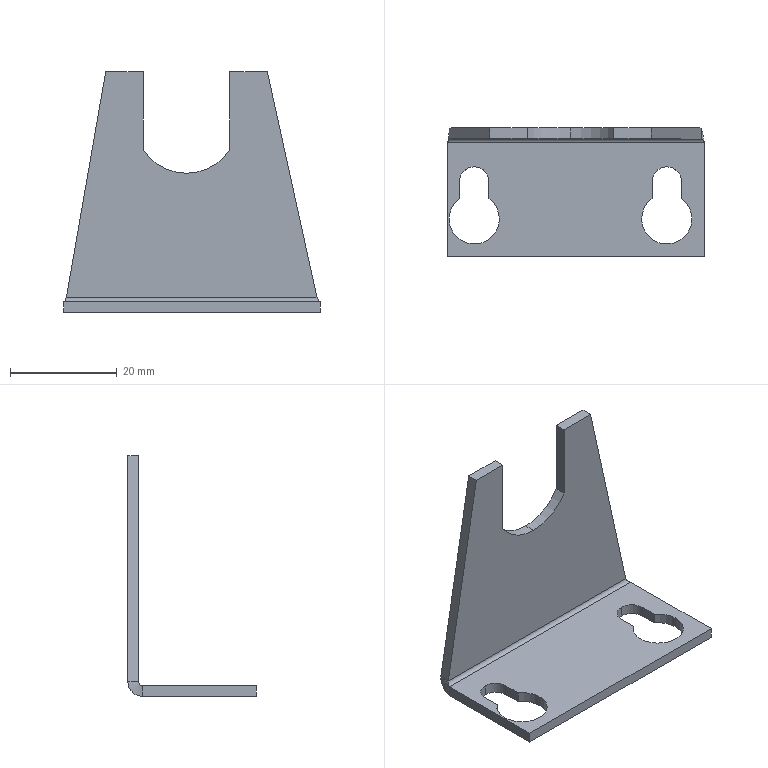Part | SolidWorks | features BaseBody 1 | 1 solid | 29 faces | box 47.946 x 24 x 45 mm | volume 4600 mm3 | plane 17 | cylinder 10 | spline 2 | commonest cylinder face diameters 5.5 x4 9.4 x2 19.08 x2 1.473 x1 5.473 x1
STEP:
#1=CARTESIAN_POINT('',(0.,2.,-10.682));
#2=VERTEX_POINT('',#1);
#3=CARTESIAN_POINT('',(8.1,2.,-6.182));
#4=VERTEX_POINT('',#3);
#5=CARTESIAN_POINT('',(0.,2.,-1.142));
#6=DIRECTION('',(0.,-1.,0.));
#7=DIRECTION('',(0.,0.,-1.));
#8=AXIS2_PLACEMENT_3D('',#5,#6,#7);
#9=CIRCLE('',#8,9.54);
#10=EDGE_CURVE('',#2,#4,#9,.T.);
#11=ORIENTED_EDGE('',*,*,#10,.F.);
#12=CARTESIAN_POINT('',(0.,0.,-10.682));
#13=VERTEX_POINT('',#12);
#14=CARTESIAN_POINT('',(0.,2.,-10.682));
#15=DIRECTION('',(0.,-1.,0.));
#16=VECTOR('',#15,1000.);
#17=LINE('',#14,#16);
#18=EDGE_CURVE('',#2,#13,#17,.T.);
#19=ORIENTED_EDGE('',*,*,#18,.T.);
#20=CARTESIAN_POINT('',(8.1,0.,-6.182));
#21=VERTEX_POINT('',#20);
#22=CARTESIAN_POINT('',(0.,0.,-1.142));
#23=DIRECTION('',(0.,1.,0.));
#24=DIRECTION('',(0.,0.,-1.));
#25=AXIS2_PLACEMENT_3D('',#22,#23,#24);
#26=CIRCLE('',#25,9.54);
#27=EDGE_CURVE('',#21,#13,#26,.T.);
#28=ORIENTED_EDGE('',*,*,#27,.F.);
#29=CARTESIAN_POINT('',(8.1,2.,-6.182));
#30=DIRECTION('',(0.,-1.,0.));
#31=VECTOR('',#30,1000.);
#32=LINE('',#29,#31);
#33=EDGE_CURVE('',#4,#21,#32,.T.);
#34=ORIENTED_EDGE('',*,*,#33,.F.);
#35=EDGE_LOOP('',(#11,#19,#28,#34));
#36=FACE_OUTER_BOUND('',#35,.T.);
#37=CARTESIAN_POINT('',(0.,2.,-1.142));
#38=DIRECTION('',(0.,-1.,0.));
#39=DIRECTION('',(0.,0.,-1.));
#40=AXIS2_PLACEMENT_3D('',#37,#38,#39);
#41=CYLINDRICAL_SURFACE('',#40,9.54);
#42=ADVANCED_FACE('',(#36),#41,.F.);
#43=CARTESIAN_POINT('',(-15.25,-8.,-34.682));
#44=VERTEX_POINT('',#43);
#45=CARTESIAN_POINT('',(-18.,-5.25,-34.682));
#46=VERTEX_POINT('',#45);
#47=CARTESIAN_POINT('',(-18.,-8.,-34.682));
#48=DIRECTION('',(0.,0.,1.));
#49=DIRECTION('',(0.,1.,0.));
#50=AXIS2_PLACEMENT_3D('',#47,#48,#49);
#51=CIRCLE('',#50,2.75);
#52=EDGE_CURVE('',#44,#46,#51,.T.);
#53=ORIENTED_EDGE('',*,*,#52,.T.);
#54=CARTESIAN_POINT('',(-18.,-5.25,-36.682));
#55=VERTEX_POINT('',#54);
#56=CARTESIAN_POINT('',(-18.,-5.25,-26.682));
#57=DIRECTION('',(0.,0.,-1.));
#58=VECTOR('',#57,1000.);
#59=LINE('',#56,#58);
#60=EDGE_CURVE('',#46,#55,#59,.T.);
#61=ORIENTED_EDGE('',*,*,#60,.T.);
#62=CARTESIAN_POINT('',(-15.25,-8.,-36.682));
#63=VERTEX_POINT('',#62);
#64=CARTESIAN_POINT('',(-18.,-8.,-36.682));
#65=DIRECTION('',(0.,0.,1.));
#66=DIRECTION('',(0.,1.,0.));
#67=AXIS2_PLACEMENT_3D('',#64,#65,#66);
#68=CIRCLE('',#67,2.75);
#69=EDGE_CURVE('',#63,#55,#68,.T.);
#70=ORIENTED_EDGE('',*,*,#69,.F.);
#71=CARTESIAN_POINT('',(-15.25,-8.,-26.682));
#72=DIRECTION('',(0.,0.,1.));
#73=VECTOR('',#72,1000.);
#74=LINE('',#71,#73);
#75=EDGE_CURVE('',#63,#44,#74,.T.);
#76=ORIENTED_EDGE('',*,*,#75,.T.);
#77=EDGE_LOOP('',(#53,#61,#70,#76));
#78=FACE_OUTER_BOUND('',#77,.T.);
#79=CARTESIAN_POINT('',(-18.,-8.,-26.682));
#80=DIRECTION('',(0.,0.,-1.));
#81=DIRECTION('',(0.,1.,0.));
#82=AXIS2_PLACEMENT_3D('',#79,#80,#81);
#83=CYLINDRICAL_SURFACE('',#82,2.75);
#84=ADVANCED_FACE('',(#78),#83,.F.);
#85=CARTESIAN_POINT('',(20.75,-8.,-34.682));
#86=VERTEX_POINT('',#85);
#87=CARTESIAN_POINT('',(18.,-5.25,-34.682));
#88=VERTEX_POINT('',#87);
#89=CARTESIAN_POINT('',(18.,-8.,-34.682));
#90=DIRECTION('',(0.,0.,1.));
#91=DIRECTION('',(0.,1.,0.));
#92=AXIS2_PLACEMENT_3D('',#89,#90,#91);
#93=CIRCLE('',#92,2.75);
#94=EDGE_CURVE('',#86,#88,#93,.T.);
#95=ORIENTED_EDGE('',*,*,#94,.T.);
#96=CARTESIAN_POINT('',(18.,-5.25,-36.682));
#97=VERTEX_POINT('',#96);
#98=CARTESIAN_POINT('',(18.,-5.25,-26.682));
#99=DIRECTION('',(0.,0.,-1.));
#100=VECTOR('',#99,1000.);
#101=LINE('',#98,#100);
#102=EDGE_CURVE('',#88,#97,#101,.T.);
#103=ORIENTED_EDGE('',*,*,#102,.T.);
#104=CARTESIAN_POINT('',(20.75,-8.,-36.682));
#105=VERTEX_POINT('',#104);
#106=CARTESIAN_POINT('',(18.,-8.,-36.682));
#107=DIRECTION('',(0.,0.,1.));
#108=DIRECTION('',(0.,1.,0.));
#109=AXIS2_PLACEMENT_3D('',#106,#107,#108);
#110=CIRCLE('',#109,2.75);
#111=EDGE_CURVE('',#105,#97,#110,.T.);
#112=ORIENTED_EDGE('',*,*,#111,.F.);
#113=CARTESIAN_POINT('',(20.75,-8.,-26.682));
#114=DIRECTION('',(0.,0.,1.));
#115=VECTOR('',#114,1000.);
#116=LINE('',#113,#115);
#117=EDGE_CURVE('',#105,#86,#116,.T.);
#118=ORIENTED_EDGE('',*,*,#117,.T.);
#119=EDGE_LOOP('',(#95,#103,#112,#118));
#120=FACE_OUTER_BOUND('',#119,.T.);
#121=CARTESIAN_POINT('',(18.,-8.,-26.682));
#122=DIRECTION('',(0.,0.,-1.));
#123=DIRECTION('',(0.,1.,0.));
#124=AXIS2_PLACEMENT_3D('',#121,#122,#123);
#125=CYLINDRICAL_SURFACE('',#124,2.75);
#126=ADVANCED_FACE('',(#120),#125,.F.);
#127=ORIENTED_EDGE('',*,*,#111,.T.);
#128=CARTESIAN_POINT('',(15.25,-8.,-36.682));
#129=VERTEX_POINT('',#128);
#130=CARTESIAN_POINT('',(18.,-8.,-36.682));
#131=DIRECTION('',(0.,0.,1.));
#132=DIRECTION('',(0.,1.,0.));
#133=AXIS2_PLACEMENT_3D('',#130,#131,#132);
#134=CIRCLE('',#133,2.75);
#135=EDGE_CURVE('',#97,#129,#134,.T.);
#136=ORIENTED_EDGE('',*,*,#135,.T.);
#137=CARTESIAN_POINT('',(15.25,-11.189,-36.682));
#138=VERTEX_POINT('',#137);
#139=CARTESIAN_POINT('',(15.25,-8.,-36.682));
#140=DIRECTION('',(0.,-1.,0.));
#141=VECTOR('',#140,1000.);
#142=LINE('',#139,#141);
#143=EDGE_CURVE('',#129,#138,#142,.T.);
#144=ORIENTED_EDGE('',*,*,#143,.T.);
#145=CARTESIAN_POINT('',(20.75,-11.189,-36.682));
#146=VERTEX_POINT('',#145);
#147=CARTESIAN_POINT('',(18.,-15.,-36.682));
#148=DIRECTION('',(0.,0.,1.));
#149=DIRECTION('',(0.,1.,0.));
#150=AXIS2_PLACEMENT_3D('',#147,#148,#149);
#151=CIRCLE('',#150,4.7);
#152=EDGE_CURVE('',#138,#146,#151,.T.);
#153=ORIENTED_EDGE('',*,*,#152,.T.);
#154=CARTESIAN_POINT('',(20.75,-8.,-36.682));
#155=DIRECTION('',(0.,1.,0.));
#156=VECTOR('',#155,1000.);
#157=LINE('',#154,#156);
#158=EDGE_CURVE('',#146,#105,#157,.T.);
#159=ORIENTED_EDGE('',*,*,#158,.T.);
#160=EDGE_LOOP('',(#127,#136,#144,#153,#159));
#161=FACE_BOUND('',#160,.T.);
#162=ORIENTED_EDGE('',*,*,#69,.T.);
#163=CARTESIAN_POINT('',(-20.75,-8.,-36.682));
#164=VERTEX_POINT('',#163);
#165=CARTESIAN_POINT('',(-18.,-8.,-36.682));
#166=DIRECTION('',(0.,0.,1.));
#167=DIRECTION('',(0.,1.,0.));
#168=AXIS2_PLACEMENT_3D('',#165,#166,#167);
#169=CIRCLE('',#168,2.75);
#170=EDGE_CURVE('',#55,#164,#169,.T.);
#171=ORIENTED_EDGE('',*,*,#170,.T.);
#172=CARTESIAN_POINT('',(-20.75,-11.189,-36.682));
#173=VERTEX_POINT('',#172);
#174=CARTESIAN_POINT('',(-20.75,-8.,-36.682));
#175=DIRECTION('',(0.,-1.,0.));
#176=VECTOR('',#175,1000.);
#177=LINE('',#174,#176);
#178=EDGE_CURVE('',#164,#173,#177,.T.);
#179=ORIENTED_EDGE('',*,*,#178,.T.);
#180=CARTESIAN_POINT('',(-15.25,-11.189,-36.682));
#181=VERTEX_POINT('',#180);
#182=CARTESIAN_POINT('',(-18.,-15.,-36.682));
#183=DIRECTION('',(0.,0.,1.));
#184=DIRECTION('',(0.,1.,0.));
#185=AXIS2_PLACEMENT_3D('',#182,#183,#184);
#186=CIRCLE('',#185,4.7);
#187=EDGE_CURVE('',#173,#181,#186,.T.);
#188=ORIENTED_EDGE('',*,*,#187,.T.);
#189=CARTESIAN_POINT('',(-15.25,-8.,-36.682));
#190=DIRECTION('',(0.,1.,0.));
#191=VECTOR('',#190,1000.);
#192=LINE('',#189,#191);
#193=EDGE_CURVE('',#181,#63,#192,.T.);
#194=ORIENTED_EDGE('',*,*,#193,.T.);
#195=EDGE_LOOP('',(#162,#171,#179,#188,#194));
#196=FACE_BOUND('',#195,.T.);
#197=CARTESIAN_POINT('',(25.,-22.,-36.682));
#198=VERTEX_POINT('',#197);
#199=CARTESIAN_POINT('',(25.,-0.7366,-36.682));
#200=VERTEX_POINT('',#199);
#201=CARTESIAN_POINT('',(25.,0.,-36.682));
#202=DIRECTION('',(0.,1.,0.));
#203=VECTOR('',#202,1000.);
#204=LINE('',#201,#203);
#205=EDGE_CURVE('',#198,#200,#204,.T.);
#206=ORIENTED_EDGE('',*,*,#205,.F.);
#207=CARTESIAN_POINT('',(-22.946,-22.,-36.682));
#208=VERTEX_POINT('',#207);
#209=CARTESIAN_POINT('',(25.,-22.,-36.682));
#210=DIRECTION('',(1.,0.,0.));
#211=VECTOR('',#210,1000.);
#212=LINE('',#209,#211);
#213=EDGE_CURVE('',#208,#198,#212,.T.);
#214=ORIENTED_EDGE('',*,*,#213,.F.);
#215=CARTESIAN_POINT('',(-22.946,-0.7366,-36.682));
#216=VERTEX_POINT('',#215);
#217=CARTESIAN_POINT('',(-22.946,-22.,-36.682));
#218=DIRECTION('',(0.,-1.,0.));
#219=VECTOR('',#218,1000.);
#220=LINE('',#217,#219);
#221=EDGE_CURVE('',#216,#208,#220,.T.);
#222=ORIENTED_EDGE('',*,*,#221,.F.);
#223=CARTESIAN_POINT('',(25.,-0.7366,-36.682));
#224=DIRECTION('',(-1.,0.,0.));
#225=VECTOR('',#224,1000.);
#226=LINE('',#223,#225);
#227=EDGE_CURVE('',#200,#216,#226,.T.);
#228=ORIENTED_EDGE('',*,*,#227,.F.);
#229=EDGE_LOOP('',(#206,#214,#222,#228));
#230=FACE_OUTER_BOUND('',#229,.T.);
#231=CARTESIAN_POINT('',(25.,0.,-36.682));
#232=DIRECTION('',(0.,0.,-1.));
#233=DIRECTION('',(-1.,0.,0.));
#234=AXIS2_PLACEMENT_3D('',#231,#232,#233);
#235=PLANE('',#234);
#236=ADVANCED_FACE('',(#161,#196,#230),#235,.T.);
#237=ORIENTED_EDGE('',*,*,#143,.F.);
#238=CARTESIAN_POINT('',(15.25,-8.,-34.682));
#239=VERTEX_POINT('',#238);
#240=CARTESIAN_POINT('',(15.25,-8.,-26.682));
#241=DIRECTION('',(0.,0.,-1.));
#242=VECTOR('',#241,1000.);
#243=LINE('',#240,#242);
#244=EDGE_CURVE('',#239,#129,#243,.T.);
#245=ORIENTED_EDGE('',*,*,#244,.F.);
#246=CARTESIAN_POINT('',(15.25,-11.189,-34.682));
#247=VERTEX_POINT('',#246);
#248=CARTESIAN_POINT('',(15.25,0.,-34.682));
#249=DIRECTION('',(0.,-1.,0.));
#250=VECTOR('',#249,1000.);
#251=LINE('',#248,#250);
#252=EDGE_CURVE('',#239,#247,#251,.T.);
#253=ORIENTED_EDGE('',*,*,#252,.T.);
#254=CARTESIAN_POINT('',(15.25,-11.189,-26.682));
#255=DIRECTION('',(0.,0.,-1.));
#256=VECTOR('',#255,1000.);
#257=LINE('',#254,#256);
#258=EDGE_CURVE('',#247,#138,#257,.T.);
#259=ORIENTED_EDGE('',*,*,#258,.T.);
#260=EDGE_LOOP('',(#237,#245,#253,#259));
#261=FACE_OUTER_BOUND('',#260,.T.);
#262=CARTESIAN_POINT('',(15.25,-8.,-26.682));
#263=DIRECTION('',(-1.,0.,0.));
#264=DIRECTION('',(0.,1.,0.));
#265=AXIS2_PLACEMENT_3D('',#262,#263,#264);
#266=PLANE('',#265);
#267=ADVANCED_FACE('',(#261),#266,.F.);
#268=ORIENTED_EDGE('',*,*,#152,.F.);
#269=ORIENTED_EDGE('',*,*,#258,.F.);
#270=CARTESIAN_POINT('',(20.75,-11.189,-34.682));
#271=VERTEX_POINT('',#270);
#272=CARTESIAN_POINT('',(18.,-15.,-34.682));
#273=DIRECTION('',(0.,0.,1.));
#274=DIRECTION('',(0.,1.,0.));
#275=AXIS2_PLACEMENT_3D('',#272,#273,#274);
#276=CIRCLE('',#275,4.7);
#277=EDGE_CURVE('',#247,#271,#276,.T.);
#278=ORIENTED_EDGE('',*,*,#277,.T.);
#279=CARTESIAN_POINT('',(20.75,-11.189,-26.682));
#280=DIRECTION('',(0.,0.,-1.));
#281=VECTOR('',#280,1000.);
#282=LINE('',#279,#281);
#283=EDGE_CURVE('',#271,#146,#282,.T.);
#284=ORIENTED_EDGE('',*,*,#283,.T.);
#285=EDGE_LOOP('',(#268,#269,#278,#284));
#286=FACE_OUTER_BOUND('',#285,.T.);
#287=CARTESIAN_POINT('',(18.,-15.,-26.682));
#288=DIRECTION('',(0.,0.,-1.));
#289=DIRECTION('',(0.,1.,0.));
#290=AXIS2_PLACEMENT_3D('',#287,#288,#289);
#291=CYLINDRICAL_SURFACE('',#290,4.7);
#292=ADVANCED_FACE('',(#286),#291,.F.);
#293=ORIENTED_EDGE('',*,*,#158,.F.);
#294=ORIENTED_EDGE('',*,*,#283,.F.);
#295=CARTESIAN_POINT('',(20.75,0.,-34.682));
#296=DIRECTION('',(0.,1.,0.));
#297=VECTOR('',#296,1000.);
#298=LINE('',#295,#297);
#299=EDGE_CURVE('',#271,#86,#298,.T.);
#300=ORIENTED_EDGE('',*,*,#299,.T.);
#301=ORIENTED_EDGE('',*,*,#117,.F.);
#302=EDGE_LOOP('',(#293,#294,#300,#301));
#303=FACE_OUTER_BOUND('',#302,.T.);
#304=CARTESIAN_POINT('',(20.75,-8.,-26.682));
#305=DIRECTION('',(1.,0.,0.));
#306=DIRECTION('',(0.,0.,-1.));
#307=AXIS2_PLACEMENT_3D('',#304,#305,#306);
#308=PLANE('',#307);
#309=ADVANCED_FACE('',(#303),#308,.F.);
#310=ORIENTED_EDGE('',*,*,#178,.F.);
#311=CARTESIAN_POINT('',(-20.75,-8.,-34.682));
#312=VERTEX_POINT('',#311);
#313=CARTESIAN_POINT('',(-20.75,-8.,-26.682));
#314=DIRECTION('',(0.,0.,-1.));
#315=VECTOR('',#314,1000.);
#316=LINE('',#313,#315);
#317=EDGE_CURVE('',#312,#164,#316,.T.);
#318=ORIENTED_EDGE('',*,*,#317,.F.);
#319=CARTESIAN_POINT('',(-20.75,-11.189,-34.682));
#320=VERTEX_POINT('',#319);
#321=CARTESIAN_POINT('',(-20.75,0.,-34.682));
#322=DIRECTION('',(0.,-1.,0.));
#323=VECTOR('',#322,1000.);
#324=LINE('',#321,#323);
#325=EDGE_CURVE('',#312,#320,#324,.T.);
#326=ORIENTED_EDGE('',*,*,#325,.T.);
#327=CARTESIAN_POINT('',(-20.75,-11.189,-26.682));
#328=DIRECTION('',(0.,0.,-1.));
#329=VECTOR('',#328,1000.);
#330=LINE('',#327,#329);
#331=EDGE_CURVE('',#320,#173,#330,.T.);
#332=ORIENTED_EDGE('',*,*,#331,.T.);
#333=EDGE_LOOP('',(#310,#318,#326,#332));
#334=FACE_OUTER_BOUND('',#333,.T.);
#335=CARTESIAN_POINT('',(-20.75,-8.,-26.682));
#336=DIRECTION('',(-1.,0.,0.));
#337=DIRECTION('',(0.,1.,0.));
#338=AXIS2_PLACEMENT_3D('',#335,#336,#337);
#339=PLANE('',#338);
#340=ADVANCED_FACE('',(#334),#339,.F.);
#341=ORIENTED_EDGE('',*,*,#187,.F.);
#342=ORIENTED_EDGE('',*,*,#331,.F.);
#343=CARTESIAN_POINT('',(-15.25,-11.189,-34.682));
#344=VERTEX_POINT('',#343);
#345=CARTESIAN_POINT('',(-18.,-15.,-34.682));
#346=DIRECTION('',(0.,0.,1.));
#347=DIRECTION('',(0.,1.,0.));
#348=AXIS2_PLACEMENT_3D('',#345,#346,#347);
#349=CIRCLE('',#348,4.7);
#350=EDGE_CURVE('',#320,#344,#349,.T.);
#351=ORIENTED_EDGE('',*,*,#350,.T.);
#352=CARTESIAN_POINT('',(-15.25,-11.189,-26.682));
#353=DIRECTION('',(0.,0.,-1.));
#354=VECTOR('',#353,1000.);
#355=LINE('',#352,#354);
#356=EDGE_CURVE('',#344,#181,#355,.T.);
#357=ORIENTED_EDGE('',*,*,#356,.T.);
#358=EDGE_LOOP('',(#341,#342,#351,#357));
#359=FACE_OUTER_BOUND('',#358,.T.);
#360=CARTESIAN_POINT('',(-18.,-15.,-26.682));
#361=DIRECTION('',(0.,0.,-1.));
#362=DIRECTION('',(0.,1.,0.));
#363=AXIS2_PLACEMENT_3D('',#360,#361,#362);
#364=CYLINDRICAL_SURFACE('',#363,4.7);
#365=ADVANCED_FACE('',(#359),#364,.F.);
#366=ORIENTED_EDGE('',*,*,#193,.F.);
#367=ORIENTED_EDGE('',*,*,#356,.F.);
#368=CARTESIAN_POINT('',(-15.25,0.,-34.682));
#369=DIRECTION('',(0.,1.,0.));
#370=VECTOR('',#369,1000.);
#371=LINE('',#368,#370);
#372=EDGE_CURVE('',#344,#44,#371,.T.);
#373=ORIENTED_EDGE('',*,*,#372,.T.);
#374=ORIENTED_EDGE('',*,*,#75,.F.);
#375=EDGE_LOOP('',(#366,#367,#373,#374));
#376=FACE_OUTER_BOUND('',#375,.T.);
#377=CARTESIAN_POINT('',(-15.25,-8.,-26.682));
#378=DIRECTION('',(1.,0.,0.));
#379=DIRECTION('',(0.,0.,-1.));
#380=AXIS2_PLACEMENT_3D('',#377,#378,#379);
#381=PLANE('',#380);
#382=ADVANCED_FACE('',(#376),#381,.F.);
#383=ORIENTED_EDGE('',*,*,#213,.T.);
#384=CARTESIAN_POINT('',(25.,-22.,-34.682));
#385=VERTEX_POINT('',#384);
#386=CARTESIAN_POINT('',(25.,-22.,-36.682));
#387=DIRECTION('',(0.,0.,-1.));
#388=VECTOR('',#387,1000.);
#389=LINE('',#386,#388);
#390=EDGE_CURVE('',#385,#198,#389,.T.);
#391=ORIENTED_EDGE('',*,*,#390,.F.);
#392=CARTESIAN_POINT('',(-22.946,-22.,-34.682));
#393=VERTEX_POINT('',#392);
#394=CARTESIAN_POINT('',(25.,-22.,-34.682));
#395=DIRECTION('',(-1.,0.,0.));
#396=VECTOR('',#395,1000.);
#397=LINE('',#394,#396);
#398=EDGE_CURVE('',#385,#393,#397,.T.);
#399=ORIENTED_EDGE('',*,*,#398,.T.);
#400=CARTESIAN_POINT('',(-22.946,-22.,-36.682));
#401=DIRECTION('',(0.,0.,1.));
#402=VECTOR('',#401,1000.);
#403=LINE('',#400,#402);
#404=EDGE_CURVE('',#208,#393,#403,.T.);
#405=ORIENTED_EDGE('',*,*,#404,.F.);
#406=EDGE_LOOP('',(#383,#391,#399,#405));
#407=FACE_OUTER_BOUND('',#406,.T.);
#408=CARTESIAN_POINT('',(25.,-22.,-36.682));
#409=DIRECTION('',(0.,-1.,0.));
#410=DIRECTION('',(0.,0.,-1.));
#411=AXIS2_PLACEMENT_3D('',#408,#409,#410);
#412=PLANE('',#411);
#413=ADVANCED_FACE('',(#407),#412,.T.);
#414=ORIENTED_EDGE('',*,*,#221,.T.);
#415=ORIENTED_EDGE('',*,*,#404,.T.);
#416=CARTESIAN_POINT('',(-22.946,-0.7366,-34.682));
#417=VERTEX_POINT('',#416);
#418=CARTESIAN_POINT('',(-22.946,0.,-34.682));
#419=DIRECTION('',(0.,1.,0.));
#420=VECTOR('',#419,1000.);
#421=LINE('',#418,#420);
#422=EDGE_CURVE('',#393,#417,#421,.T.);
#423=ORIENTED_EDGE('',*,*,#422,.T.);
#424=CARTESIAN_POINT('',(-22.946,-0.7366,-35.682));
#425=DIRECTION('',(0.,0.,-1.));
#426=VECTOR('',#425,1000.);
#427=LINE('',#424,#426);
#428=EDGE_CURVE('',#417,#216,#427,.T.);
#429=ORIENTED_EDGE('',*,*,#428,.T.);
#430=EDGE_LOOP('',(#414,#415,#423,#429));
#431=FACE_OUTER_BOUND('',#430,.T.);
#432=CARTESIAN_POINT('',(-22.946,-22.,-36.682));
#433=DIRECTION('',(-1.,0.,0.));
#434=DIRECTION('',(0.,1.,0.));
#435=AXIS2_PLACEMENT_3D('',#432,#433,#434);
#436=PLANE('',#435);
#437=ADVANCED_FACE('',(#431),#436,.T.);
#438=CARTESIAN_POINT('',(25.,-0.7366,-34.682));
#439=VERTEX_POINT('',#438);
#440=CARTESIAN_POINT('',(25.,0.,-34.682));
#441=DIRECTION('',(0.,-1.,0.));
#442=VECTOR('',#441,1000.);
#443=LINE('',#440,#442);
#444=EDGE_CURVE('',#439,#385,#443,.T.);
#445=ORIENTED_EDGE('',*,*,#444,.T.);
#446=ORIENTED_EDGE('',*,*,#390,.T.);
#447=ORIENTED_EDGE('',*,*,#205,.T.);
#448=CARTESIAN_POINT('',(25.,-0.7366,-35.682));
#449=DIRECTION('',(0.,0.,1.));
#450=VECTOR('',#449,1000.);
#451=LINE('',#448,#450);
#452=EDGE_CURVE('',#200,#439,#451,.T.);
#453=ORIENTED_EDGE('',*,*,#452,.T.);
#454=EDGE_LOOP('',(#445,#446,#447,#453));
#455=FACE_OUTER_BOUND('',#454,.T.);
#456=CARTESIAN_POINT('',(25.,0.,-36.682));
#457=DIRECTION('',(1.,0.,0.));
#458=DIRECTION('',(0.,0.,-1.));
#459=AXIS2_PLACEMENT_3D('',#456,#457,#458);
#460=PLANE('',#459);
#461=ADVANCED_FACE('',(#455),#460,.T.);
#462=ORIENTED_EDGE('',*,*,#227,.T.);
#463=CARTESIAN_POINT('',(-22.469,2.,-33.946));
#464=VERTEX_POINT('',#463);
#465=CARTESIAN_POINT('',(-22.946,-0.7366,-36.682));
#466=CARTESIAN_POINT('',(-22.906,-0.3784,-36.682));
#467=CARTESIAN_POINT('',(-22.867,-0.0203,-36.611));
#468=CARTESIAN_POINT('',(-22.787,0.6416,-36.337));
#469=CARTESIAN_POINT('',(-22.747,0.9452,-36.134));
#470=CARTESIAN_POINT('',(-22.668,1.452,-35.628));
#471=CARTESIAN_POINT('',(-22.628,1.655,-35.324));
#472=CARTESIAN_POINT('',(-22.549,1.929,-34.662));
#473=CARTESIAN_POINT('',(-22.509,2.,-34.304));
#474=CARTESIAN_POINT('',(-22.469,2.,-33.946));
#475=B_SPLINE_CURVE_WITH_KNOTS('',3,(#465,#466,#467,#468,#469,#470,#471,#472,#473,#474),.UNSPECIFIED.,.F.,.F.,(4,2,2,2,4),(0.,0.25,0.5,0.75,1.),.UNSPECIFIED.);
#476=EDGE_CURVE('',#216,#464,#475,.T.);
#477=ORIENTED_EDGE('',*,*,#476,.T.);
#478=CARTESIAN_POINT('',(24.398,2.,-33.946));
#479=VERTEX_POINT('',#478);
#480=CARTESIAN_POINT('',(0.,2.,-33.946));
#481=DIRECTION('',(1.,0.,0.));
#482=VECTOR('',#481,1000.);
#483=LINE('',#480,#482);
#484=EDGE_CURVE('',#464,#479,#483,.T.);
#485=ORIENTED_EDGE('',*,*,#484,.T.);
#486=CARTESIAN_POINT('',(24.398,2.,-33.946));
#487=CARTESIAN_POINT('',(24.449,2.,-34.307));
#488=CARTESIAN_POINT('',(24.498,1.93,-34.657));
#489=CARTESIAN_POINT('',(24.573,1.724,-35.158));
#490=CARTESIAN_POINT('',(24.598,1.64,-35.315));
#491=CARTESIAN_POINT('',(24.648,1.442,-35.612));
#492=CARTESIAN_POINT('',(24.674,1.327,-35.753));
#493=CARTESIAN_POINT('',(24.724,1.073,-36.006));
#494=CARTESIAN_POINT('',(24.749,0.9356,-36.119));
#495=CARTESIAN_POINT('',(24.799,0.6384,-36.319));
#496=CARTESIAN_POINT('',(24.824,0.4778,-36.405));
#497=CARTESIAN_POINT('',(24.899,-0.01677,-36.61));
#498=CARTESIAN_POINT('',(24.949,-0.375,-36.682));
#499=CARTESIAN_POINT('',(25.,-0.7366,-36.682));
#500=B_SPLINE_CURVE_WITH_KNOTS('',3,(#486,#487,#488,#489,#490,#491,#492,#493,#494,#495,#496,#497,#498,#499),.UNSPECIFIED.,.F.,.F.,(4,2,2,2,2,2,4),(0.,0.001076,0.001614,0.002152,0.00269,0.003228,0.004304),.UNSPECIFIED.);
#501=EDGE_CURVE('',#479,#200,#500,.T.);
#502=ORIENTED_EDGE('',*,*,#501,.T.);
#503=EDGE_LOOP('',(#462,#477,#485,#502));
#504=FACE_OUTER_BOUND('',#503,.T.);
#505=CARTESIAN_POINT('',(25.,-0.7366,-33.946));
#506=DIRECTION('',(1.,0.,0.));
#507=DIRECTION('',(0.,0.,-1.));
#508=AXIS2_PLACEMENT_3D('',#505,#506,#507);
#509=CYLINDRICAL_SURFACE('',#508,2.737);
#510=ADVANCED_FACE('',(#504),#509,.T.);
#511=CARTESIAN_POINT('',(-22.469,0.,-33.946));
#512=VERTEX_POINT('',#511);
#513=CARTESIAN_POINT('',(-22.469,0.,-33.946));
#514=CARTESIAN_POINT('',(-22.549,0.,-34.139));
#515=CARTESIAN_POINT('',(-22.628,-0.07939,-34.33));
#516=CARTESIAN_POINT('',(-22.787,-0.3521,-34.603));
#517=CARTESIAN_POINT('',(-22.867,-0.5438,-34.682));
#518=CARTESIAN_POINT('',(-22.946,-0.7366,-34.682));
#519=B_SPLINE_CURVE_WITH_KNOTS('',3,(#513,#514,#515,#516,#517,#518),.UNSPECIFIED.,.F.,.F.,(4,2,4),(0.,0.5,1.),.UNSPECIFIED.);
#520=EDGE_CURVE('',#512,#417,#519,.T.);
#521=ORIENTED_EDGE('',*,*,#520,.F.);
#522=CARTESIAN_POINT('',(-22.469,2.,-33.946));
#523=DIRECTION('',(0.,1.,0.));
#524=VECTOR('',#523,1000.);
#525=LINE('',#522,#524);
#526=EDGE_CURVE('',#512,#464,#525,.T.);
#527=ORIENTED_EDGE('',*,*,#526,.T.);
#528=ORIENTED_EDGE('',*,*,#476,.F.);
#529=ORIENTED_EDGE('',*,*,#428,.F.);
#530=EDGE_LOOP('',(#521,#527,#528,#529));
#531=FACE_OUTER_BOUND('',#530,.T.);
#532=CARTESIAN_POINT('',(-22.469,2.02,-33.946));
#533=CARTESIAN_POINT('',(-22.509,2.02,-34.307));
#534=CARTESIAN_POINT('',(-22.549,1.948,-34.667));
#535=CARTESIAN_POINT('',(-22.628,1.672,-35.334));
#536=CARTESIAN_POINT('',(-22.668,1.468,-35.64));
#537=CARTESIAN_POINT('',(-22.747,0.9575,-36.15));
#538=CARTESIAN_POINT('',(-22.787,0.6517,-36.354));
#539=CARTESIAN_POINT('',(-22.867,-0.01507,-36.631));
#540=CARTESIAN_POINT('',(-22.906,-0.3757,-36.702));
#541=CARTESIAN_POINT('',(-22.946,-0.7366,-36.702));
#542=CARTESIAN_POINT('',(-22.469,2.,-33.946));
#543=CARTESIAN_POINT('',(-22.509,2.,-34.304));
#544=CARTESIAN_POINT('',(-22.549,1.929,-34.662));
#545=CARTESIAN_POINT('',(-22.628,1.655,-35.324));
#546=CARTESIAN_POINT('',(-22.668,1.452,-35.628));
#547=CARTESIAN_POINT('',(-22.747,0.9452,-36.134));
#548=CARTESIAN_POINT('',(-22.787,0.6416,-36.337));
#549=CARTESIAN_POINT('',(-22.867,-0.0203,-36.611));
#550=CARTESIAN_POINT('',(-22.906,-0.3783,-36.682));
#551=CARTESIAN_POINT('',(-22.946,-0.7366,-36.682));
#552=CARTESIAN_POINT('',(-22.469,0.,-33.946));
#553=CARTESIAN_POINT('',(-22.509,0.,-34.042));
#554=CARTESIAN_POINT('',(-22.549,-0.01917,-34.139));
#555=CARTESIAN_POINT('',(-22.628,-0.09297,-34.317));
#556=CARTESIAN_POINT('',(-22.668,-0.1476,-34.398));
#557=CARTESIAN_POINT('',(-22.747,-0.2839,-34.535));
#558=CARTESIAN_POINT('',(-22.787,-0.3656,-34.589));
#559=CARTESIAN_POINT('',(-22.867,-0.5438,-34.663));
#560=CARTESIAN_POINT('',(-22.906,-0.6402,-34.682));
#561=CARTESIAN_POINT('',(-22.946,-0.7366,-34.682));
#562=CARTESIAN_POINT('',(-22.469,-0.0202,-33.946));
#563=CARTESIAN_POINT('',(-22.509,-0.0202,-34.04));
#564=CARTESIAN_POINT('',(-22.549,-0.03885,-34.133));
#565=CARTESIAN_POINT('',(-22.628,-0.1106,-34.307));
#566=CARTESIAN_POINT('',(-22.668,-0.1637,-34.386));
#567=CARTESIAN_POINT('',(-22.747,-0.2963,-34.519));
#568=CARTESIAN_POINT('',(-22.787,-0.3758,-34.572));
#569=CARTESIAN_POINT('',(-22.867,-0.5491,-34.644));
#570=CARTESIAN_POINT('',(-22.906,-0.6428,-34.662));
#571=CARTESIAN_POINT('',(-22.946,-0.7366,-34.662));
#572=B_SPLINE_SURFACE_WITH_KNOTS('',1,3,((#532,#533,#534,#535,#536,#537,#538,#539,#540,#541),(#542,#543,#544,#545,#546,#547,#548,#549,#550,#551),(#552,#553,#554,#555,#556,#557,#558,#559,#560,#561),(#562,#563,#564,#565,#566,#567,#568,#569,#570,#571)),.UNSPECIFIED.,.F.,.F.,.F.,(2,1,1,2),(4,2,2,2,4),(-0.01,0.,1.,1.01),(0.,0.25,0.5,0.75,1.),.UNSPECIFIED.);
#573=ADVANCED_FACE('',(#531),#572,.F.);
#574=ORIENTED_EDGE('',*,*,#277,.F.);
#575=ORIENTED_EDGE('',*,*,#252,.F.);
#576=CARTESIAN_POINT('',(18.,-8.,-34.682));
#577=DIRECTION('',(0.,0.,1.));
#578=DIRECTION('',(0.,1.,0.));
#579=AXIS2_PLACEMENT_3D('',#576,#577,#578);
#580=CIRCLE('',#579,2.75);
#581=EDGE_CURVE('',#88,#239,#580,.T.);
#582=ORIENTED_EDGE('',*,*,#581,.F.);
#583=ORIENTED_EDGE('',*,*,#94,.F.);
#584=ORIENTED_EDGE('',*,*,#299,.F.);
#585=EDGE_LOOP('',(#574,#575,#582,#583,#584));
#586=FACE_BOUND('',#585,.T.);
#587=ORIENTED_EDGE('',*,*,#350,.F.);
#588=ORIENTED_EDGE('',*,*,#325,.F.);
#589=CARTESIAN_POINT('',(-18.,-8.,-34.682));
#590=DIRECTION('',(0.,0.,1.));
#591=DIRECTION('',(0.,1.,0.));
#592=AXIS2_PLACEMENT_3D('',#589,#590,#591);
#593=CIRCLE('',#592,2.75);
#594=EDGE_CURVE('',#46,#312,#593,.T.);
#595=ORIENTED_EDGE('',*,*,#594,.F.);
#596=ORIENTED_EDGE('',*,*,#52,.F.);
#597=ORIENTED_EDGE('',*,*,#372,.F.);
#598=EDGE_LOOP('',(#587,#588,#595,#596,#597));
#599=FACE_BOUND('',#598,.T.);
#600=ORIENTED_EDGE('',*,*,#422,.F.);
#601=ORIENTED_EDGE('',*,*,#398,.F.);
#602=ORIENTED_EDGE('',*,*,#444,.F.);
#603=CARTESIAN_POINT('',(25.,-0.7366,-34.682));
#604=DIRECTION('',(-1.,0.,0.));
#605=VECTOR('',#604,1000.);
#606=LINE('',#603,#605);
#607=EDGE_CURVE('',#439,#417,#606,.T.);
#608=ORIENTED_EDGE('',*,*,#607,.T.);
#609=EDGE_LOOP('',(#600,#601,#602,#608));
#610=FACE_OUTER_BOUND('',#609,.T.);
#611=CARTESIAN_POINT('',(25.,0.,-34.682));
#612=DIRECTION('',(0.,0.,-1.));
#613=DIRECTION('',(-1.,0.,0.));
#614=AXIS2_PLACEMENT_3D('',#611,#612,#613);
#615=PLANE('',#614);
#616=ADVANCED_FACE('',(#586,#599,#610),#615,.F.);
#617=ORIENTED_EDGE('',*,*,#452,.F.);
#618=ORIENTED_EDGE('',*,*,#501,.F.);
#619=CARTESIAN_POINT('',(24.398,0.,-33.946));
#620=VERTEX_POINT('',#619);
#621=CARTESIAN_POINT('',(24.398,2.,-33.946));
#622=DIRECTION('',(0.,-1.,0.));
#623=VECTOR('',#622,1000.);
#624=LINE('',#621,#623);
#625=EDGE_CURVE('',#479,#620,#624,.T.);
#626=ORIENTED_EDGE('',*,*,#625,.T.);
#627=CARTESIAN_POINT('',(24.398,0.,-33.946));
#628=CARTESIAN_POINT('',(24.498,0.,-34.139));
#629=CARTESIAN_POINT('',(24.599,-0.07939,-34.33));
#630=CARTESIAN_POINT('',(24.799,-0.3521,-34.603));
#631=CARTESIAN_POINT('',(24.9,-0.5438,-34.682));
#632=CARTESIAN_POINT('',(25.,-0.7366,-34.682));
#633=B_SPLINE_CURVE_WITH_KNOTS('',3,(#627,#628,#629,#630,#631,#632),.UNSPECIFIED.,.F.,.F.,(4,2,4),(0.,0.5,1.),.UNSPECIFIED.);
#634=EDGE_CURVE('',#620,#439,#633,.T.);
#635=ORIENTED_EDGE('',*,*,#634,.T.);
#636=EDGE_LOOP('',(#617,#618,#626,#635));
#637=FACE_OUTER_BOUND('',#636,.T.);
#638=CARTESIAN_POINT('',(25.,-0.7366,-36.702));
#639=CARTESIAN_POINT('',(24.95,-0.3757,-36.702));
#640=CARTESIAN_POINT('',(24.9,-0.01507,-36.631));
#641=CARTESIAN_POINT('',(24.799,0.6517,-36.354));
#642=CARTESIAN_POINT('',(24.749,0.9575,-36.15));
#643=CARTESIAN_POINT('',(24.649,1.468,-35.64));
#644=CARTESIAN_POINT('',(24.599,1.672,-35.334));
#645=CARTESIAN_POINT('',(24.498,1.948,-34.667));
#646=CARTESIAN_POINT('',(24.448,2.02,-34.307));
#647=CARTESIAN_POINT('',(24.398,2.02,-33.946));
#648=CARTESIAN_POINT('',(25.,-0.7366,-36.682));
#649=CARTESIAN_POINT('',(24.95,-0.3783,-36.682));
#650=CARTESIAN_POINT('',(24.9,-0.0203,-36.611));
#651=CARTESIAN_POINT('',(24.799,0.6416,-36.337));
#652=CARTESIAN_POINT('',(24.749,0.9452,-36.134));
#653=CARTESIAN_POINT('',(24.649,1.452,-35.628));
#654=CARTESIAN_POINT('',(24.599,1.655,-35.324));
#655=CARTESIAN_POINT('',(24.498,1.929,-34.662));
#656=CARTESIAN_POINT('',(24.448,2.,-34.304));
#657=CARTESIAN_POINT('',(24.398,2.,-33.946));
#658=CARTESIAN_POINT('',(25.,-0.7366,-34.682));
#659=CARTESIAN_POINT('',(24.95,-0.6402,-34.682));
#660=CARTESIAN_POINT('',(24.9,-0.5438,-34.663));
#661=CARTESIAN_POINT('',(24.799,-0.3656,-34.589));
#662=CARTESIAN_POINT('',(24.749,-0.2839,-34.535));
#663=CARTESIAN_POINT('',(24.649,-0.1476,-34.398));
#664=CARTESIAN_POINT('',(24.599,-0.09297,-34.317));
#665=CARTESIAN_POINT('',(24.498,-0.01917,-34.139));
#666=CARTESIAN_POINT('',(24.448,0.,-34.042));
#667=CARTESIAN_POINT('',(24.398,0.,-33.946));
#668=CARTESIAN_POINT('',(25.,-0.7366,-34.662));
#669=CARTESIAN_POINT('',(24.95,-0.6428,-34.662));
#670=CARTESIAN_POINT('',(24.9,-0.5491,-34.644));
#671=CARTESIAN_POINT('',(24.799,-0.3758,-34.572));
#672=CARTESIAN_POINT('',(24.749,-0.2963,-34.519));
#673=CARTESIAN_POINT('',(24.649,-0.1637,-34.386));
#674=CARTESIAN_POINT('',(24.599,-0.1106,-34.307));
#675=CARTESIAN_POINT('',(24.498,-0.03885,-34.133));
#676=CARTESIAN_POINT('',(24.448,-0.0202,-34.04));
#677=CARTESIAN_POINT('',(24.398,-0.0202,-33.946));
#678=B_SPLINE_SURFACE_WITH_KNOTS('',1,3,((#638,#639,#640,#641,#642,#643,#644,#645,#646,#647),(#648,#649,#650,#651,#652,#653,#654,#655,#656,#657),(#658,#659,#660,#661,#662,#663,#664,#665,#666,#667),(#668,#669,#670,#671,#672,#673,#674,#675,#676,#677)),.UNSPECIFIED.,.F.,.F.,.F.,(2,1,1,2),(4,2,2,2,4),(-0.01,0.,1.,1.01),(0.,0.25,0.5,0.75,1.),.UNSPECIFIED.);
#679=ADVANCED_FACE('',(#637),#678,.F.);
#680=CARTESIAN_POINT('',(-15.1,2.,8.318));
#681=VERTEX_POINT('',#680);
#682=CARTESIAN_POINT('',(-22.946,2.,-36.682));
#683=DIRECTION('',(0.1718,0.,0.9851));
#684=VECTOR('',#683,1000.);
#685=LINE('',#682,#684);
#686=EDGE_CURVE('',#464,#681,#685,.T.);
#687=ORIENTED_EDGE('',*,*,#686,.T.);
#688=CARTESIAN_POINT('',(-8.1,2.,8.318));
#689=VERTEX_POINT('',#688);
#690=CARTESIAN_POINT('',(-8.1,2.,8.318));
#691=DIRECTION('',(1.,0.,0.));
#692=VECTOR('',#691,1000.);
#693=LINE('',#690,#692);
#694=EDGE_CURVE('',#681,#689,#693,.T.);
#695=ORIENTED_EDGE('',*,*,#694,.T.);
#696=CARTESIAN_POINT('',(-8.1,2.,-6.182));
#697=VERTEX_POINT('',#696);
#698=CARTESIAN_POINT('',(-8.1,2.,-6.182));
#699=DIRECTION('',(0.,0.,-1.));
#700=VECTOR('',#699,1000.);
#701=LINE('',#698,#700);
#702=EDGE_CURVE('',#689,#697,#701,.T.);
#703=ORIENTED_EDGE('',*,*,#702,.T.);
#704=CARTESIAN_POINT('',(0.,2.,-1.142));
#705=DIRECTION('',(0.,-1.,0.));
#706=DIRECTION('',(0.,0.,-1.));
#707=AXIS2_PLACEMENT_3D('',#704,#705,#706);
#708=CIRCLE('',#707,9.54);
#709=EDGE_CURVE('',#697,#2,#708,.T.);
#710=ORIENTED_EDGE('',*,*,#709,.T.);
#711=ORIENTED_EDGE('',*,*,#10,.T.);
#712=CARTESIAN_POINT('',(8.1,2.,8.318));
#713=VERTEX_POINT('',#712);
#714=CARTESIAN_POINT('',(8.1,2.,8.318));
#715=DIRECTION('',(0.,0.,1.));
#716=VECTOR('',#715,1000.);
#717=LINE('',#714,#716);
#718=EDGE_CURVE('',#4,#713,#717,.T.);
#719=ORIENTED_EDGE('',*,*,#718,.T.);
#720=CARTESIAN_POINT('',(15.1,2.,8.318));
#721=VERTEX_POINT('',#720);
#722=CARTESIAN_POINT('',(8.1,2.,8.318));
#723=DIRECTION('',(1.,0.,0.));
#724=VECTOR('',#723,1000.);
#725=LINE('',#722,#724);
#726=EDGE_CURVE('',#713,#721,#725,.T.);
#727=ORIENTED_EDGE('',*,*,#726,.T.);
#728=CARTESIAN_POINT('',(15.1,2.,8.318));
#729=DIRECTION('',(0.2149,0.,-0.9766));
#730=VECTOR('',#729,1000.);
#731=LINE('',#728,#730);
#732=EDGE_CURVE('',#721,#479,#731,.T.);
#733=ORIENTED_EDGE('',*,*,#732,.T.);
#734=ORIENTED_EDGE('',*,*,#484,.F.);
#735=EDGE_LOOP('',(#687,#695,#703,#710,#711,#719,#727,#733,#734));
#736=FACE_OUTER_BOUND('',#735,.T.);
#737=CARTESIAN_POINT('',(0.,2.,-1.142));
#738=DIRECTION('',(0.,-1.,0.));
#739=DIRECTION('',(0.,0.,-1.));
#740=AXIS2_PLACEMENT_3D('',#737,#738,#739);
#741=PLANE('',#740);
#742=ADVANCED_FACE('',(#736),#741,.F.);
#743=CARTESIAN_POINT('',(-15.1,0.,8.318));
#744=VERTEX_POINT('',#743);
#745=CARTESIAN_POINT('',(-15.1,0.,8.318));
#746=DIRECTION('',(-0.1718,0.,-0.9851));
#747=VECTOR('',#746,1000.);
#748=LINE('',#745,#747);
#749=EDGE_CURVE('',#744,#512,#748,.T.);
#750=ORIENTED_EDGE('',*,*,#749,.F.);
#751=CARTESIAN_POINT('',(-15.1,2.,8.318));
#752=DIRECTION('',(0.,1.,0.));
#753=VECTOR('',#752,1000.);
#754=LINE('',#751,#753);
#755=EDGE_CURVE('',#744,#681,#754,.T.);
#756=ORIENTED_EDGE('',*,*,#755,.T.);
#757=ORIENTED_EDGE('',*,*,#686,.F.);
#758=ORIENTED_EDGE('',*,*,#526,.F.);
#759=EDGE_LOOP('',(#750,#756,#757,#758));
#760=FACE_OUTER_BOUND('',#759,.T.);
#761=CARTESIAN_POINT('',(-22.946,2.,-36.682));
#762=DIRECTION('',(0.9851,0.,-0.1718));
#763=DIRECTION('',(0.,-1.,0.));
#764=AXIS2_PLACEMENT_3D('',#761,#762,#763);
#765=PLANE('',#764);
#766=ADVANCED_FACE('',(#760),#765,.F.);
#767=ORIENTED_EDGE('',*,*,#520,.T.);
#768=ORIENTED_EDGE('',*,*,#607,.F.);
#769=ORIENTED_EDGE('',*,*,#634,.F.);
#770=CARTESIAN_POINT('',(0.,0.,-33.946));
#771=DIRECTION('',(1.,0.,0.));
#772=VECTOR('',#771,1000.);
#773=LINE('',#770,#772);
#774=EDGE_CURVE('',#512,#620,#773,.T.);
#775=ORIENTED_EDGE('',*,*,#774,.F.);
#776=EDGE_LOOP('',(#767,#768,#769,#775));
#777=FACE_OUTER_BOUND('',#776,.T.);
#778=CARTESIAN_POINT('',(25.,-0.7366,-33.946));
#779=DIRECTION('',(1.,0.,0.));
#780=DIRECTION('',(0.,0.,-1.));
#781=AXIS2_PLACEMENT_3D('',#778,#779,#780);
#782=CYLINDRICAL_SURFACE('',#781,0.7366);
#783=ADVANCED_FACE('',(#777),#782,.F.);
#784=ORIENTED_EDGE('',*,*,#732,.F.);
#785=CARTESIAN_POINT('',(15.1,0.,8.318));
#786=VERTEX_POINT('',#785);
#787=CARTESIAN_POINT('',(15.1,2.,8.318));
#788=DIRECTION('',(0.,-1.,0.));
#789=VECTOR('',#788,1000.);
#790=LINE('',#787,#789);
#791=EDGE_CURVE('',#721,#786,#790,.T.);
#792=ORIENTED_EDGE('',*,*,#791,.T.);
#793=CARTESIAN_POINT('',(24.398,0.,-33.946));
#794=DIRECTION('',(-0.2149,0.,0.9766));
#795=VECTOR('',#794,1000.);
#796=LINE('',#793,#795);
#797=EDGE_CURVE('',#620,#786,#796,.T.);
#798=ORIENTED_EDGE('',*,*,#797,.F.);
#799=ORIENTED_EDGE('',*,*,#625,.F.);
#800=EDGE_LOOP('',(#784,#792,#798,#799));
#801=FACE_OUTER_BOUND('',#800,.T.);
#802=CARTESIAN_POINT('',(15.1,2.,8.318));
#803=DIRECTION('',(-0.9766,0.,-0.2149));
#804=DIRECTION('',(-0.2149,0.,0.9766));
#805=AXIS2_PLACEMENT_3D('',#802,#803,#804);
#806=PLANE('',#805);
#807=ADVANCED_FACE('',(#801),#806,.F.);
#808=ORIENTED_EDGE('',*,*,#791,.F.);
#809=ORIENTED_EDGE('',*,*,#726,.F.);
#810=CARTESIAN_POINT('',(8.1,0.,8.318));
#811=VERTEX_POINT('',#810);
#812=CARTESIAN_POINT('',(8.1,2.,8.318));
#813=DIRECTION('',(0.,-1.,0.));
#814=VECTOR('',#813,1000.);
#815=LINE('',#812,#814);
#816=EDGE_CURVE('',#713,#811,#815,.T.);
#817=ORIENTED_EDGE('',*,*,#816,.T.);
#818=CARTESIAN_POINT('',(0.,0.,8.318));
#819=DIRECTION('',(-1.,0.,0.));
#820=VECTOR('',#819,1000.);
#821=LINE('',#818,#820);
#822=EDGE_CURVE('',#786,#811,#821,.T.);
#823=ORIENTED_EDGE('',*,*,#822,.F.);
#824=EDGE_LOOP('',(#808,#809,#817,#823));
#825=FACE_OUTER_BOUND('',#824,.T.);
#826=CARTESIAN_POINT('',(8.1,2.,8.318));
#827=DIRECTION('',(0.,0.,-1.));
#828=DIRECTION('',(0.,-1.,0.));
#829=AXIS2_PLACEMENT_3D('',#826,#827,#828);
#830=PLANE('',#829);
#831=ADVANCED_FACE('',(#825),#830,.F.);
#832=ORIENTED_EDGE('',*,*,#816,.F.);
#833=ORIENTED_EDGE('',*,*,#718,.F.);
#834=ORIENTED_EDGE('',*,*,#33,.T.);
#835=CARTESIAN_POINT('',(8.1,0.,-1.142));
#836=DIRECTION('',(0.,0.,-1.));
#837=VECTOR('',#836,1000.);
#838=LINE('',#835,#837);
#839=EDGE_CURVE('',#811,#21,#838,.T.);
#840=ORIENTED_EDGE('',*,*,#839,.F.);
#841=EDGE_LOOP('',(#832,#833,#834,#840));
#842=FACE_OUTER_BOUND('',#841,.T.);
#843=CARTESIAN_POINT('',(8.1,2.,8.318));
#844=DIRECTION('',(1.,0.,0.));
#845=DIRECTION('',(0.,1.,0.));
#846=AXIS2_PLACEMENT_3D('',#843,#844,#845);
#847=PLANE('',#846);
#848=ADVANCED_FACE('',(#842),#847,.F.);
#849=CARTESIAN_POINT('',(-8.1,0.,-6.182));
#850=VERTEX_POINT('',#849);
#851=CARTESIAN_POINT('',(-8.1,2.,-6.182));
#852=DIRECTION('',(0.,-1.,0.));
#853=VECTOR('',#852,1000.);
#854=LINE('',#851,#853);
#855=EDGE_CURVE('',#697,#850,#854,.T.);
#856=ORIENTED_EDGE('',*,*,#855,.F.);
#857=ORIENTED_EDGE('',*,*,#702,.F.);
#858=CARTESIAN_POINT('',(-8.1,0.,8.318));
#859=VERTEX_POINT('',#858);
#860=CARTESIAN_POINT('',(-8.1,2.,8.318));
#861=DIRECTION('',(0.,-1.,0.));
#862=VECTOR('',#861,1000.);
#863=LINE('',#860,#862);
#864=EDGE_CURVE('',#689,#859,#863,.T.);
#865=ORIENTED_EDGE('',*,*,#864,.T.);
#866=CARTESIAN_POINT('',(-8.1,0.,-1.142));
#867=DIRECTION('',(0.,0.,1.));
#868=VECTOR('',#867,1000.);
#869=LINE('',#866,#868);
#870=EDGE_CURVE('',#850,#859,#869,.T.);
#871=ORIENTED_EDGE('',*,*,#870,.F.);
#872=EDGE_LOOP('',(#856,#857,#865,#871));
#873=FACE_OUTER_BOUND('',#872,.T.);
#874=CARTESIAN_POINT('',(-8.1,2.,-6.182));
#875=DIRECTION('',(-1.,0.,0.));
#876=DIRECTION('',(0.,0.,1.));
#877=AXIS2_PLACEMENT_3D('',#874,#875,#876);
#878=PLANE('',#877);
#879=ADVANCED_FACE('',(#873),#878,.F.);
#880=ORIENTED_EDGE('',*,*,#864,.F.);
#881=ORIENTED_EDGE('',*,*,#694,.F.);
#882=ORIENTED_EDGE('',*,*,#755,.F.);
#883=CARTESIAN_POINT('',(0.,0.,8.318));
#884=DIRECTION('',(-1.,0.,0.));
#885=VECTOR('',#884,1000.);
#886=LINE('',#883,#885);
#887=EDGE_CURVE('',#859,#744,#886,.T.);
#888=ORIENTED_EDGE('',*,*,#887,.F.);
#889=EDGE_LOOP('',(#880,#881,#882,#888));
#890=FACE_OUTER_BOUND('',#889,.T.);
#891=CARTESIAN_POINT('',(-8.1,2.,8.318));
#892=DIRECTION('',(0.,0.,-1.));
#893=DIRECTION('',(0.,-1.,0.));
#894=AXIS2_PLACEMENT_3D('',#891,#892,#893);
#895=PLANE('',#894);
#896=ADVANCED_FACE('',(#890),#895,.F.);
#897=ORIENTED_EDGE('',*,*,#870,.T.);
#898=ORIENTED_EDGE('',*,*,#887,.T.);
#899=ORIENTED_EDGE('',*,*,#749,.T.);
#900=ORIENTED_EDGE('',*,*,#774,.T.);
#901=ORIENTED_EDGE('',*,*,#797,.T.);
#902=ORIENTED_EDGE('',*,*,#822,.T.);
#903=ORIENTED_EDGE('',*,*,#839,.T.);
#904=ORIENTED_EDGE('',*,*,#27,.T.);
#905=CARTESIAN_POINT('',(0.,0.,-1.142));
#906=DIRECTION('',(0.,1.,0.));
#907=DIRECTION('',(0.,0.,-1.));
#908=AXIS2_PLACEMENT_3D('',#905,#906,#907);
#909=CIRCLE('',#908,9.54);
#910=EDGE_CURVE('',#13,#850,#909,.T.);
#911=ORIENTED_EDGE('',*,*,#910,.T.);
#912=EDGE_LOOP('',(#897,#898,#899,#900,#901,#902,#903,#904,#911));
#913=FACE_OUTER_BOUND('',#912,.T.);
#914=CARTESIAN_POINT('',(0.,0.,-1.142));
#915=DIRECTION('',(0.,-1.,0.));
#916=DIRECTION('',(0.,0.,-1.));
#917=AXIS2_PLACEMENT_3D('',#914,#915,#916);
#918=PLANE('',#917);
#919=ADVANCED_FACE('',(#913),#918,.T.);
#920=ORIENTED_EDGE('',*,*,#102,.F.);
#921=ORIENTED_EDGE('',*,*,#581,.T.);
#922=ORIENTED_EDGE('',*,*,#244,.T.);
#923=ORIENTED_EDGE('',*,*,#135,.F.);
#924=EDGE_LOOP('',(#920,#921,#922,#923));
#925=FACE_OUTER_BOUND('',#924,.T.);
#926=CARTESIAN_POINT('',(18.,-8.,-26.682));
#927=DIRECTION('',(0.,0.,-1.));
#928=DIRECTION('',(0.,1.,0.));
#929=AXIS2_PLACEMENT_3D('',#926,#927,#928);
#930=CYLINDRICAL_SURFACE('',#929,2.75);
#931=ADVANCED_FACE('',(#925),#930,.F.);
#932=ORIENTED_EDGE('',*,*,#60,.F.);
#933=ORIENTED_EDGE('',*,*,#594,.T.);
#934=ORIENTED_EDGE('',*,*,#317,.T.);
#935=ORIENTED_EDGE('',*,*,#170,.F.);
#936=EDGE_LOOP('',(#932,#933,#934,#935));
#937=FACE_OUTER_BOUND('',#936,.T.);
#938=CARTESIAN_POINT('',(-18.,-8.,-26.682));
#939=DIRECTION('',(0.,0.,-1.));
#940=DIRECTION('',(0.,1.,0.));
#941=AXIS2_PLACEMENT_3D('',#938,#939,#940);
#942=CYLINDRICAL_SURFACE('',#941,2.75);
#943=ADVANCED_FACE('',(#937),#942,.F.);
#944=ORIENTED_EDGE('',*,*,#18,.F.);
#945=ORIENTED_EDGE('',*,*,#709,.F.);
#946=ORIENTED_EDGE('',*,*,#855,.T.);
#947=ORIENTED_EDGE('',*,*,#910,.F.);
#948=EDGE_LOOP('',(#944,#945,#946,#947));
#949=FACE_OUTER_BOUND('',#948,.T.);
#950=CARTESIAN_POINT('',(0.,2.,-1.142));
#951=DIRECTION('',(0.,-1.,0.));
#952=DIRECTION('',(0.,0.,-1.));
#953=AXIS2_PLACEMENT_3D('',#950,#951,#952);
#954=CYLINDRICAL_SURFACE('',#953,9.54);
#955=ADVANCED_FACE('',(#949),#954,.F.);
#956=CLOSED_SHELL('',(#42,#84,#126,#236,#267,#292,#309,#340,#365,#382,#413,#437,#461,#510,#573,#616,#679,#742,#766,#783,#807,#831,#848,#879,#896,#919,#931,#943,#955));
#957=MANIFOLD_SOLID_BREP('',#956);
#958=CARTESIAN_POINT('',(0.,0.,0.));
#959=DIRECTION('',(0.,0.,1.));
#960=DIRECTION('',(1.,0.,0.));
#961=AXIS2_PLACEMENT_3D('',#958,#959,#960);
#962=(LENGTH_UNIT()NAMED_UNIT(*)SI_UNIT(.MILLI.,.METRE.));
#963=UNCERTAINTY_MEASURE_WITH_UNIT(LENGTH_MEASURE(0.00001),#962,'','');
#964=(NAMED_UNIT(*)PLANE_ANGLE_UNIT()SI_UNIT($,.RADIAN.));
#965=(NAMED_UNIT(*)SI_UNIT($,.STERADIAN.)SOLID_ANGLE_UNIT());
#966=(GEOMETRIC_REPRESENTATION_CONTEXT(3)GLOBAL_UNCERTAINTY_ASSIGNED_CONTEXT((#963))GLOBAL_UNIT_ASSIGNED_CONTEXT((#962,#964,#965))REPRESENTATION_CONTEXT('',''));
#967=ADVANCED_BREP_SHAPE_REPRESENTATION('',(#957,#961),#966);